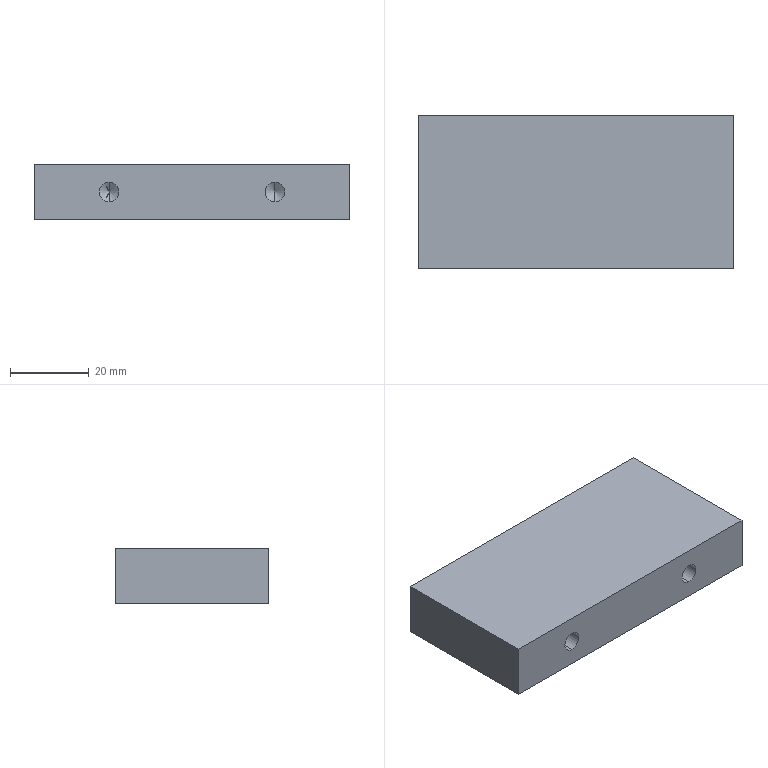Part | SolidWorks | features HoleWzd 2, Extrusion 1 | 1 solid | 22 faces | box 80 x 39 x 14 mm | volume 42305 mm3 | cylinder 8 | cone 8 | plane 6 | commonest cylinder face diameters 5 x8
STEP:
#1=CARTESIAN_POINT('',(-33.,2.5,4.5));
#2=VERTEX_POINT('',#1);
#3=CARTESIAN_POINT('',(-33.,2.5,9.5));
#4=VERTEX_POINT('',#3);
#5=CARTESIAN_POINT('',(-33.,2.5,7.));
#6=DIRECTION('',(0.,1.,0.));
#7=DIRECTION('',(0.,0.,1.));
#8=AXIS2_PLACEMENT_3D('',#5,#6,#7);
#9=CIRCLE('',#8,2.5);
#10=EDGE_CURVE('',#2,#4,#9,.T.);
#11=ORIENTED_EDGE('',*,*,#10,.F.);
#12=CARTESIAN_POINT('',(-33.,19.5,4.5));
#13=VERTEX_POINT('',#12);
#14=CARTESIAN_POINT('',(-33.,19.5,4.5));
#15=DIRECTION('',(0.,1.,0.));
#16=VECTOR('',#15,1000.);
#17=LINE('',#14,#16);
#18=EDGE_CURVE('',#2,#13,#17,.T.);
#19=ORIENTED_EDGE('',*,*,#18,.T.);
#20=CARTESIAN_POINT('',(-33.,19.5,9.5));
#21=VERTEX_POINT('',#20);
#22=CARTESIAN_POINT('',(-33.,19.5,7.));
#23=DIRECTION('',(0.,1.,0.));
#24=DIRECTION('',(0.,0.,1.));
#25=AXIS2_PLACEMENT_3D('',#22,#23,#24);
#26=CIRCLE('',#25,2.5);
#27=EDGE_CURVE('',#13,#21,#26,.T.);
#28=ORIENTED_EDGE('',*,*,#27,.T.);
#29=CARTESIAN_POINT('',(-33.,19.5,9.5));
#30=DIRECTION('',(0.,1.,0.));
#31=VECTOR('',#30,1000.);
#32=LINE('',#29,#31);
#33=EDGE_CURVE('',#4,#21,#32,.T.);
#34=ORIENTED_EDGE('',*,*,#33,.F.);
#35=EDGE_LOOP('',(#11,#19,#28,#34));
#36=FACE_OUTER_BOUND('',#35,.T.);
#37=CARTESIAN_POINT('',(-33.,19.5,7.));
#38=DIRECTION('',(0.,1.,0.));
#39=DIRECTION('',(0.,0.,1.));
#40=AXIS2_PLACEMENT_3D('',#37,#38,#39);
#41=CYLINDRICAL_SURFACE('',#40,2.5);
#42=ADVANCED_FACE('',(#36),#41,.F.);
#43=CARTESIAN_POINT('',(-33.,0.9978,7.));
#44=VERTEX_POINT('',#43);
#45=CARTESIAN_POINT('',(-33.,2.5,9.5));
#46=DIRECTION('',(0.,0.515,0.8572));
#47=VECTOR('',#46,1000.);
#48=LINE('',#45,#47);
#49=EDGE_CURVE('',#44,#4,#48,.T.);
#50=ORIENTED_EDGE('',*,*,#49,.F.);
#51=CARTESIAN_POINT('',(-33.,2.5,4.5));
#52=DIRECTION('',(0.,0.515,-0.8572));
#53=VECTOR('',#52,1000.);
#54=LINE('',#51,#53);
#55=EDGE_CURVE('',#44,#2,#54,.T.);
#56=ORIENTED_EDGE('',*,*,#55,.T.);
#57=ORIENTED_EDGE('',*,*,#10,.T.);
#58=EDGE_LOOP('',(#50,#56,#57));
#59=FACE_OUTER_BOUND('',#58,.T.);
#60=CARTESIAN_POINT('',(-33.,2.5,7.));
#61=DIRECTION('',(0.,1.,0.));
#62=DIRECTION('',(0.,0.,1.));
#63=AXIS2_PLACEMENT_3D('',#60,#61,#62);
#64=CONICAL_SURFACE('',#63,2.5,1.03);
#65=ADVANCED_FACE('',(#59),#64,.F.);
#66=CARTESIAN_POINT('',(33.,2.5,4.5));
#67=VERTEX_POINT('',#66);
#68=CARTESIAN_POINT('',(33.,2.5,9.5));
#69=VERTEX_POINT('',#68);
#70=CARTESIAN_POINT('',(33.,2.5,7.));
#71=DIRECTION('',(0.,1.,0.));
#72=DIRECTION('',(0.,0.,1.));
#73=AXIS2_PLACEMENT_3D('',#70,#71,#72);
#74=CIRCLE('',#73,2.5);
#75=EDGE_CURVE('',#67,#69,#74,.T.);
#76=ORIENTED_EDGE('',*,*,#75,.F.);
#77=CARTESIAN_POINT('',(33.,19.5,4.5));
#78=VERTEX_POINT('',#77);
#79=CARTESIAN_POINT('',(33.,19.5,4.5));
#80=DIRECTION('',(0.,1.,0.));
#81=VECTOR('',#80,1000.);
#82=LINE('',#79,#81);
#83=EDGE_CURVE('',#67,#78,#82,.T.);
#84=ORIENTED_EDGE('',*,*,#83,.T.);
#85=CARTESIAN_POINT('',(33.,19.5,9.5));
#86=VERTEX_POINT('',#85);
#87=CARTESIAN_POINT('',(33.,19.5,7.));
#88=DIRECTION('',(0.,1.,0.));
#89=DIRECTION('',(0.,0.,1.));
#90=AXIS2_PLACEMENT_3D('',#87,#88,#89);
#91=CIRCLE('',#90,2.5);
#92=EDGE_CURVE('',#78,#86,#91,.T.);
#93=ORIENTED_EDGE('',*,*,#92,.T.);
#94=CARTESIAN_POINT('',(33.,19.5,9.5));
#95=DIRECTION('',(0.,1.,0.));
#96=VECTOR('',#95,1000.);
#97=LINE('',#94,#96);
#98=EDGE_CURVE('',#69,#86,#97,.T.);
#99=ORIENTED_EDGE('',*,*,#98,.F.);
#100=EDGE_LOOP('',(#76,#84,#93,#99));
#101=FACE_OUTER_BOUND('',#100,.T.);
#102=CARTESIAN_POINT('',(33.,19.5,7.));
#103=DIRECTION('',(0.,1.,0.));
#104=DIRECTION('',(0.,0.,1.));
#105=AXIS2_PLACEMENT_3D('',#102,#103,#104);
#106=CYLINDRICAL_SURFACE('',#105,2.5);
#107=ADVANCED_FACE('',(#101),#106,.F.);
#108=CARTESIAN_POINT('',(33.,0.9978,7.));
#109=VERTEX_POINT('',#108);
#110=CARTESIAN_POINT('',(33.,2.5,9.5));
#111=DIRECTION('',(0.,0.515,0.8572));
#112=VECTOR('',#111,1000.);
#113=LINE('',#110,#112);
#114=EDGE_CURVE('',#109,#69,#113,.T.);
#115=ORIENTED_EDGE('',*,*,#114,.F.);
#116=CARTESIAN_POINT('',(33.,2.5,4.5));
#117=DIRECTION('',(0.,0.515,-0.8572));
#118=VECTOR('',#117,1000.);
#119=LINE('',#116,#118);
#120=EDGE_CURVE('',#109,#67,#119,.T.);
#121=ORIENTED_EDGE('',*,*,#120,.T.);
#122=ORIENTED_EDGE('',*,*,#75,.T.);
#123=EDGE_LOOP('',(#115,#121,#122));
#124=FACE_OUTER_BOUND('',#123,.T.);
#125=CARTESIAN_POINT('',(33.,2.5,7.));
#126=DIRECTION('',(0.,1.,0.));
#127=DIRECTION('',(0.,0.,1.));
#128=AXIS2_PLACEMENT_3D('',#125,#126,#127);
#129=CONICAL_SURFACE('',#128,2.5,1.03);
#130=ADVANCED_FACE('',(#124),#129,.F.);
#131=CARTESIAN_POINT('',(21.,-2.5,9.5));
#132=VERTEX_POINT('',#131);
#133=CARTESIAN_POINT('',(21.,-2.5,4.5));
#134=VERTEX_POINT('',#133);
#135=CARTESIAN_POINT('',(21.,-2.5,7.));
#136=DIRECTION('',(0.,-1.,0.));
#137=DIRECTION('',(0.,0.,-1.));
#138=AXIS2_PLACEMENT_3D('',#135,#136,#137);
#139=CIRCLE('',#138,2.5);
#140=EDGE_CURVE('',#132,#134,#139,.T.);
#141=ORIENTED_EDGE('',*,*,#140,.F.);
#142=CARTESIAN_POINT('',(21.,-19.5,9.5));
#143=VERTEX_POINT('',#142);
#144=CARTESIAN_POINT('',(21.,-19.5,9.5));
#145=DIRECTION('',(0.,-1.,0.));
#146=VECTOR('',#145,1000.);
#147=LINE('',#144,#146);
#148=EDGE_CURVE('',#132,#143,#147,.T.);
#149=ORIENTED_EDGE('',*,*,#148,.T.);
#150=CARTESIAN_POINT('',(21.,-19.5,4.5));
#151=VERTEX_POINT('',#150);
#152=CARTESIAN_POINT('',(21.,-19.5,7.));
#153=DIRECTION('',(0.,-1.,0.));
#154=DIRECTION('',(0.,0.,-1.));
#155=AXIS2_PLACEMENT_3D('',#152,#153,#154);
#156=CIRCLE('',#155,2.5);
#157=EDGE_CURVE('',#143,#151,#156,.T.);
#158=ORIENTED_EDGE('',*,*,#157,.T.);
#159=CARTESIAN_POINT('',(21.,-19.5,4.5));
#160=DIRECTION('',(0.,-1.,0.));
#161=VECTOR('',#160,1000.);
#162=LINE('',#159,#161);
#163=EDGE_CURVE('',#134,#151,#162,.T.);
#164=ORIENTED_EDGE('',*,*,#163,.F.);
#165=EDGE_LOOP('',(#141,#149,#158,#164));
#166=FACE_OUTER_BOUND('',#165,.T.);
#167=CARTESIAN_POINT('',(21.,-19.5,7.));
#168=DIRECTION('',(0.,-1.,0.));
#169=DIRECTION('',(0.,0.,-1.));
#170=AXIS2_PLACEMENT_3D('',#167,#168,#169);
#171=CYLINDRICAL_SURFACE('',#170,2.5);
#172=ADVANCED_FACE('',(#166),#171,.F.);
#173=CARTESIAN_POINT('',(21.,-0.9978,7.));
#174=VERTEX_POINT('',#173);
#175=CARTESIAN_POINT('',(21.,-2.5,4.5));
#176=DIRECTION('',(0.,-0.515,-0.8572));
#177=VECTOR('',#176,1000.);
#178=LINE('',#175,#177);
#179=EDGE_CURVE('',#174,#134,#178,.T.);
#180=ORIENTED_EDGE('',*,*,#179,.F.);
#181=CARTESIAN_POINT('',(21.,-2.5,9.5));
#182=DIRECTION('',(0.,-0.515,0.8572));
#183=VECTOR('',#182,1000.);
#184=LINE('',#181,#183);
#185=EDGE_CURVE('',#174,#132,#184,.T.);
#186=ORIENTED_EDGE('',*,*,#185,.T.);
#187=ORIENTED_EDGE('',*,*,#140,.T.);
#188=EDGE_LOOP('',(#180,#186,#187));
#189=FACE_OUTER_BOUND('',#188,.T.);
#190=CARTESIAN_POINT('',(21.,-2.5,7.));
#191=DIRECTION('',(0.,-1.,0.));
#192=DIRECTION('',(0.,0.,-1.));
#193=AXIS2_PLACEMENT_3D('',#190,#191,#192);
#194=CONICAL_SURFACE('',#193,2.5,1.03);
#195=ADVANCED_FACE('',(#189),#194,.F.);
#196=CARTESIAN_POINT('',(-21.,-2.5,9.5));
#197=VERTEX_POINT('',#196);
#198=CARTESIAN_POINT('',(-21.,-2.5,4.5));
#199=VERTEX_POINT('',#198);
#200=CARTESIAN_POINT('',(-21.,-2.5,7.));
#201=DIRECTION('',(0.,-1.,0.));
#202=DIRECTION('',(0.,0.,-1.));
#203=AXIS2_PLACEMENT_3D('',#200,#201,#202);
#204=CIRCLE('',#203,2.5);
#205=EDGE_CURVE('',#197,#199,#204,.T.);
#206=ORIENTED_EDGE('',*,*,#205,.F.);
#207=CARTESIAN_POINT('',(-21.,-19.5,9.5));
#208=VERTEX_POINT('',#207);
#209=CARTESIAN_POINT('',(-21.,-19.5,9.5));
#210=DIRECTION('',(0.,-1.,0.));
#211=VECTOR('',#210,1000.);
#212=LINE('',#209,#211);
#213=EDGE_CURVE('',#197,#208,#212,.T.);
#214=ORIENTED_EDGE('',*,*,#213,.T.);
#215=CARTESIAN_POINT('',(-21.,-19.5,4.5));
#216=VERTEX_POINT('',#215);
#217=CARTESIAN_POINT('',(-21.,-19.5,7.));
#218=DIRECTION('',(0.,-1.,0.));
#219=DIRECTION('',(0.,0.,-1.));
#220=AXIS2_PLACEMENT_3D('',#217,#218,#219);
#221=CIRCLE('',#220,2.5);
#222=EDGE_CURVE('',#208,#216,#221,.T.);
#223=ORIENTED_EDGE('',*,*,#222,.T.);
#224=CARTESIAN_POINT('',(-21.,-19.5,4.5));
#225=DIRECTION('',(0.,-1.,0.));
#226=VECTOR('',#225,1000.);
#227=LINE('',#224,#226);
#228=EDGE_CURVE('',#199,#216,#227,.T.);
#229=ORIENTED_EDGE('',*,*,#228,.F.);
#230=EDGE_LOOP('',(#206,#214,#223,#229));
#231=FACE_OUTER_BOUND('',#230,.T.);
#232=CARTESIAN_POINT('',(-21.,-19.5,7.));
#233=DIRECTION('',(0.,-1.,0.));
#234=DIRECTION('',(0.,0.,-1.));
#235=AXIS2_PLACEMENT_3D('',#232,#233,#234);
#236=CYLINDRICAL_SURFACE('',#235,2.5);
#237=ADVANCED_FACE('',(#231),#236,.F.);
#238=CARTESIAN_POINT('',(-21.,-0.9978,7.));
#239=VERTEX_POINT('',#238);
#240=CARTESIAN_POINT('',(-21.,-2.5,4.5));
#241=DIRECTION('',(0.,-0.515,-0.8572));
#242=VECTOR('',#241,1000.);
#243=LINE('',#240,#242);
#244=EDGE_CURVE('',#239,#199,#243,.T.);
#245=ORIENTED_EDGE('',*,*,#244,.F.);
#246=CARTESIAN_POINT('',(-21.,-2.5,9.5));
#247=DIRECTION('',(0.,-0.515,0.8572));
#248=VECTOR('',#247,1000.);
#249=LINE('',#246,#248);
#250=EDGE_CURVE('',#239,#197,#249,.T.);
#251=ORIENTED_EDGE('',*,*,#250,.T.);
#252=ORIENTED_EDGE('',*,*,#205,.T.);
#253=EDGE_LOOP('',(#245,#251,#252));
#254=FACE_OUTER_BOUND('',#253,.T.);
#255=CARTESIAN_POINT('',(-21.,-2.5,7.));
#256=DIRECTION('',(0.,-1.,0.));
#257=DIRECTION('',(0.,0.,-1.));
#258=AXIS2_PLACEMENT_3D('',#255,#256,#257);
#259=CONICAL_SURFACE('',#258,2.5,1.03);
#260=ADVANCED_FACE('',(#254),#259,.F.);
#261=CARTESIAN_POINT('',(40.,-19.5,0.));
#262=VERTEX_POINT('',#261);
#263=CARTESIAN_POINT('',(40.,19.5,0.));
#264=VERTEX_POINT('',#263);
#265=CARTESIAN_POINT('',(40.,19.5,0.));
#266=DIRECTION('',(0.,1.,0.));
#267=VECTOR('',#266,1000.);
#268=LINE('',#265,#267);
#269=EDGE_CURVE('',#262,#264,#268,.T.);
#270=ORIENTED_EDGE('',*,*,#269,.T.);
#271=CARTESIAN_POINT('',(40.,19.5,14.));
#272=VERTEX_POINT('',#271);
#273=CARTESIAN_POINT('',(40.,19.5,14.));
#274=DIRECTION('',(0.,0.,-1.));
#275=VECTOR('',#274,1000.);
#276=LINE('',#273,#275);
#277=EDGE_CURVE('',#272,#264,#276,.T.);
#278=ORIENTED_EDGE('',*,*,#277,.F.);
#279=CARTESIAN_POINT('',(40.,-19.5,14.));
#280=VERTEX_POINT('',#279);
#281=CARTESIAN_POINT('',(40.,19.5,14.));
#282=DIRECTION('',(0.,1.,0.));
#283=VECTOR('',#282,1000.);
#284=LINE('',#281,#283);
#285=EDGE_CURVE('',#280,#272,#284,.T.);
#286=ORIENTED_EDGE('',*,*,#285,.F.);
#287=CARTESIAN_POINT('',(40.,-19.5,14.));
#288=DIRECTION('',(0.,0.,-1.));
#289=VECTOR('',#288,1000.);
#290=LINE('',#287,#289);
#291=EDGE_CURVE('',#280,#262,#290,.T.);
#292=ORIENTED_EDGE('',*,*,#291,.T.);
#293=EDGE_LOOP('',(#270,#278,#286,#292));
#294=FACE_OUTER_BOUND('',#293,.T.);
#295=CARTESIAN_POINT('',(40.,19.5,14.));
#296=DIRECTION('',(-1.,0.,0.));
#297=DIRECTION('',(0.,0.,1.));
#298=AXIS2_PLACEMENT_3D('',#295,#296,#297);
#299=PLANE('',#298);
#300=ADVANCED_FACE('',(#294),#299,.F.);
#301=CARTESIAN_POINT('',(-33.,19.5,7.));
#302=DIRECTION('',(0.,1.,0.));
#303=DIRECTION('',(0.,0.,1.));
#304=AXIS2_PLACEMENT_3D('',#301,#302,#303);
#305=CIRCLE('',#304,2.5);
#306=EDGE_CURVE('',#21,#13,#305,.T.);
#307=ORIENTED_EDGE('',*,*,#306,.F.);
#308=ORIENTED_EDGE('',*,*,#27,.F.);
#309=EDGE_LOOP('',(#307,#308));
#310=FACE_BOUND('',#309,.T.);
#311=CARTESIAN_POINT('',(33.,19.5,7.));
#312=DIRECTION('',(0.,1.,0.));
#313=DIRECTION('',(0.,0.,1.));
#314=AXIS2_PLACEMENT_3D('',#311,#312,#313);
#315=CIRCLE('',#314,2.5);
#316=EDGE_CURVE('',#86,#78,#315,.T.);
#317=ORIENTED_EDGE('',*,*,#316,.F.);
#318=ORIENTED_EDGE('',*,*,#92,.F.);
#319=EDGE_LOOP('',(#317,#318));
#320=FACE_BOUND('',#319,.T.);
#321=CARTESIAN_POINT('',(-40.,19.5,0.));
#322=VERTEX_POINT('',#321);
#323=CARTESIAN_POINT('',(-40.,19.5,0.));
#324=DIRECTION('',(-1.,0.,0.));
#325=VECTOR('',#324,1000.);
#326=LINE('',#323,#325);
#327=EDGE_CURVE('',#264,#322,#326,.T.);
#328=ORIENTED_EDGE('',*,*,#327,.T.);
#329=CARTESIAN_POINT('',(-40.,19.5,14.));
#330=VERTEX_POINT('',#329);
#331=CARTESIAN_POINT('',(-40.,19.5,14.));
#332=DIRECTION('',(0.,0.,-1.));
#333=VECTOR('',#332,1000.);
#334=LINE('',#331,#333);
#335=EDGE_CURVE('',#330,#322,#334,.T.);
#336=ORIENTED_EDGE('',*,*,#335,.F.);
#337=CARTESIAN_POINT('',(-40.,19.5,14.));
#338=DIRECTION('',(-1.,0.,0.));
#339=VECTOR('',#338,1000.);
#340=LINE('',#337,#339);
#341=EDGE_CURVE('',#272,#330,#340,.T.);
#342=ORIENTED_EDGE('',*,*,#341,.F.);
#343=ORIENTED_EDGE('',*,*,#277,.T.);
#344=EDGE_LOOP('',(#328,#336,#342,#343));
#345=FACE_OUTER_BOUND('',#344,.T.);
#346=CARTESIAN_POINT('',(-40.,19.5,14.));
#347=DIRECTION('',(0.,-1.,0.));
#348=DIRECTION('',(0.,0.,-1.));
#349=AXIS2_PLACEMENT_3D('',#346,#347,#348);
#350=PLANE('',#349);
#351=ADVANCED_FACE('',(#310,#320,#345),#350,.F.);
#352=CARTESIAN_POINT('',(-40.,-19.5,0.));
#353=VERTEX_POINT('',#352);
#354=CARTESIAN_POINT('',(-40.,19.5,0.));
#355=DIRECTION('',(0.,-1.,0.));
#356=VECTOR('',#355,1000.);
#357=LINE('',#354,#356);
#358=EDGE_CURVE('',#322,#353,#357,.T.);
#359=ORIENTED_EDGE('',*,*,#358,.T.);
#360=CARTESIAN_POINT('',(-40.,-19.5,14.));
#361=VERTEX_POINT('',#360);
#362=CARTESIAN_POINT('',(-40.,-19.5,14.));
#363=DIRECTION('',(0.,0.,-1.));
#364=VECTOR('',#363,1000.);
#365=LINE('',#362,#364);
#366=EDGE_CURVE('',#361,#353,#365,.T.);
#367=ORIENTED_EDGE('',*,*,#366,.F.);
#368=CARTESIAN_POINT('',(-40.,19.5,14.));
#369=DIRECTION('',(0.,-1.,0.));
#370=VECTOR('',#369,1000.);
#371=LINE('',#368,#370);
#372=EDGE_CURVE('',#330,#361,#371,.T.);
#373=ORIENTED_EDGE('',*,*,#372,.F.);
#374=ORIENTED_EDGE('',*,*,#335,.T.);
#375=EDGE_LOOP('',(#359,#367,#373,#374));
#376=FACE_OUTER_BOUND('',#375,.T.);
#377=CARTESIAN_POINT('',(-40.,19.5,14.));
#378=DIRECTION('',(1.,0.,0.));
#379=DIRECTION('',(0.,1.,0.));
#380=AXIS2_PLACEMENT_3D('',#377,#378,#379);
#381=PLANE('',#380);
#382=ADVANCED_FACE('',(#376),#381,.F.);
#383=CARTESIAN_POINT('',(21.,-19.5,7.));
#384=DIRECTION('',(0.,-1.,0.));
#385=DIRECTION('',(0.,0.,-1.));
#386=AXIS2_PLACEMENT_3D('',#383,#384,#385);
#387=CIRCLE('',#386,2.5);
#388=EDGE_CURVE('',#151,#143,#387,.T.);
#389=ORIENTED_EDGE('',*,*,#388,.F.);
#390=ORIENTED_EDGE('',*,*,#157,.F.);
#391=EDGE_LOOP('',(#389,#390));
#392=FACE_BOUND('',#391,.T.);
#393=CARTESIAN_POINT('',(-21.,-19.5,7.));
#394=DIRECTION('',(0.,-1.,0.));
#395=DIRECTION('',(0.,0.,-1.));
#396=AXIS2_PLACEMENT_3D('',#393,#394,#395);
#397=CIRCLE('',#396,2.5);
#398=EDGE_CURVE('',#216,#208,#397,.T.);
#399=ORIENTED_EDGE('',*,*,#398,.F.);
#400=ORIENTED_EDGE('',*,*,#222,.F.);
#401=EDGE_LOOP('',(#399,#400));
#402=FACE_BOUND('',#401,.T.);
#403=CARTESIAN_POINT('',(-40.,-19.5,0.));
#404=DIRECTION('',(1.,0.,0.));
#405=VECTOR('',#404,1000.);
#406=LINE('',#403,#405);
#407=EDGE_CURVE('',#353,#262,#406,.T.);
#408=ORIENTED_EDGE('',*,*,#407,.T.);
#409=ORIENTED_EDGE('',*,*,#291,.F.);
#410=CARTESIAN_POINT('',(-40.,-19.5,14.));
#411=DIRECTION('',(1.,0.,0.));
#412=VECTOR('',#411,1000.);
#413=LINE('',#410,#412);
#414=EDGE_CURVE('',#361,#280,#413,.T.);
#415=ORIENTED_EDGE('',*,*,#414,.F.);
#416=ORIENTED_EDGE('',*,*,#366,.T.);
#417=EDGE_LOOP('',(#408,#409,#415,#416));
#418=FACE_OUTER_BOUND('',#417,.T.);
#419=CARTESIAN_POINT('',(-40.,-19.5,14.));
#420=DIRECTION('',(0.,1.,0.));
#421=DIRECTION('',(0.,0.,1.));
#422=AXIS2_PLACEMENT_3D('',#419,#420,#421);
#423=PLANE('',#422);
#424=ADVANCED_FACE('',(#392,#402,#418),#423,.F.);
#425=ORIENTED_EDGE('',*,*,#285,.T.);
#426=ORIENTED_EDGE('',*,*,#341,.T.);
#427=ORIENTED_EDGE('',*,*,#372,.T.);
#428=ORIENTED_EDGE('',*,*,#414,.T.);
#429=EDGE_LOOP('',(#425,#426,#427,#428));
#430=FACE_OUTER_BOUND('',#429,.T.);
#431=CARTESIAN_POINT('',(0.,0.,14.));
#432=DIRECTION('',(0.,0.,1.));
#433=DIRECTION('',(1.,0.,0.));
#434=AXIS2_PLACEMENT_3D('',#431,#432,#433);
#435=PLANE('',#434);
#436=ADVANCED_FACE('',(#430),#435,.T.);
#437=ORIENTED_EDGE('',*,*,#269,.F.);
#438=ORIENTED_EDGE('',*,*,#407,.F.);
#439=ORIENTED_EDGE('',*,*,#358,.F.);
#440=ORIENTED_EDGE('',*,*,#327,.F.);
#441=EDGE_LOOP('',(#437,#438,#439,#440));
#442=FACE_OUTER_BOUND('',#441,.T.);
#443=CARTESIAN_POINT('',(0.,0.,0.));
#444=DIRECTION('',(0.,0.,1.));
#445=DIRECTION('',(1.,0.,0.));
#446=AXIS2_PLACEMENT_3D('',#443,#444,#445);
#447=PLANE('',#446);
#448=ADVANCED_FACE('',(#442),#447,.F.);
#449=ORIENTED_EDGE('',*,*,#250,.F.);
#450=ORIENTED_EDGE('',*,*,#244,.T.);
#451=CARTESIAN_POINT('',(-21.,-2.5,7.));
#452=DIRECTION('',(0.,-1.,0.));
#453=DIRECTION('',(0.,0.,-1.));
#454=AXIS2_PLACEMENT_3D('',#451,#452,#453);
#455=CIRCLE('',#454,2.5);
#456=EDGE_CURVE('',#199,#197,#455,.T.);
#457=ORIENTED_EDGE('',*,*,#456,.T.);
#458=EDGE_LOOP('',(#449,#450,#457));
#459=FACE_OUTER_BOUND('',#458,.T.);
#460=CARTESIAN_POINT('',(-21.,-2.5,7.));
#461=DIRECTION('',(0.,-1.,0.));
#462=DIRECTION('',(0.,0.,-1.));
#463=AXIS2_PLACEMENT_3D('',#460,#461,#462);
#464=CONICAL_SURFACE('',#463,2.5,1.03);
#465=ADVANCED_FACE('',(#459),#464,.F.);
#466=ORIENTED_EDGE('',*,*,#213,.F.);
#467=ORIENTED_EDGE('',*,*,#456,.F.);
#468=ORIENTED_EDGE('',*,*,#228,.T.);
#469=ORIENTED_EDGE('',*,*,#398,.T.);
#470=EDGE_LOOP('',(#466,#467,#468,#469));
#471=FACE_OUTER_BOUND('',#470,.T.);
#472=CARTESIAN_POINT('',(-21.,-19.5,7.));
#473=DIRECTION('',(0.,-1.,0.));
#474=DIRECTION('',(0.,0.,-1.));
#475=AXIS2_PLACEMENT_3D('',#472,#473,#474);
#476=CYLINDRICAL_SURFACE('',#475,2.5);
#477=ADVANCED_FACE('',(#471),#476,.F.);
#478=ORIENTED_EDGE('',*,*,#185,.F.);
#479=ORIENTED_EDGE('',*,*,#179,.T.);
#480=CARTESIAN_POINT('',(21.,-2.5,7.));
#481=DIRECTION('',(0.,-1.,0.));
#482=DIRECTION('',(0.,0.,-1.));
#483=AXIS2_PLACEMENT_3D('',#480,#481,#482);
#484=CIRCLE('',#483,2.5);
#485=EDGE_CURVE('',#134,#132,#484,.T.);
#486=ORIENTED_EDGE('',*,*,#485,.T.);
#487=EDGE_LOOP('',(#478,#479,#486));
#488=FACE_OUTER_BOUND('',#487,.T.);
#489=CARTESIAN_POINT('',(21.,-2.5,7.));
#490=DIRECTION('',(0.,-1.,0.));
#491=DIRECTION('',(0.,0.,-1.));
#492=AXIS2_PLACEMENT_3D('',#489,#490,#491);
#493=CONICAL_SURFACE('',#492,2.5,1.03);
#494=ADVANCED_FACE('',(#488),#493,.F.);
#495=ORIENTED_EDGE('',*,*,#148,.F.);
#496=ORIENTED_EDGE('',*,*,#485,.F.);
#497=ORIENTED_EDGE('',*,*,#163,.T.);
#498=ORIENTED_EDGE('',*,*,#388,.T.);
#499=EDGE_LOOP('',(#495,#496,#497,#498));
#500=FACE_OUTER_BOUND('',#499,.T.);
#501=CARTESIAN_POINT('',(21.,-19.5,7.));
#502=DIRECTION('',(0.,-1.,0.));
#503=DIRECTION('',(0.,0.,-1.));
#504=AXIS2_PLACEMENT_3D('',#501,#502,#503);
#505=CYLINDRICAL_SURFACE('',#504,2.5);
#506=ADVANCED_FACE('',(#500),#505,.F.);
#507=ORIENTED_EDGE('',*,*,#120,.F.);
#508=ORIENTED_EDGE('',*,*,#114,.T.);
#509=CARTESIAN_POINT('',(33.,2.5,7.));
#510=DIRECTION('',(0.,1.,0.));
#511=DIRECTION('',(0.,0.,1.));
#512=AXIS2_PLACEMENT_3D('',#509,#510,#511);
#513=CIRCLE('',#512,2.5);
#514=EDGE_CURVE('',#69,#67,#513,.T.);
#515=ORIENTED_EDGE('',*,*,#514,.T.);
#516=EDGE_LOOP('',(#507,#508,#515));
#517=FACE_OUTER_BOUND('',#516,.T.);
#518=CARTESIAN_POINT('',(33.,2.5,7.));
#519=DIRECTION('',(0.,1.,0.));
#520=DIRECTION('',(0.,0.,1.));
#521=AXIS2_PLACEMENT_3D('',#518,#519,#520);
#522=CONICAL_SURFACE('',#521,2.5,1.03);
#523=ADVANCED_FACE('',(#517),#522,.F.);
#524=ORIENTED_EDGE('',*,*,#83,.F.);
#525=ORIENTED_EDGE('',*,*,#514,.F.);
#526=ORIENTED_EDGE('',*,*,#98,.T.);
#527=ORIENTED_EDGE('',*,*,#316,.T.);
#528=EDGE_LOOP('',(#524,#525,#526,#527));
#529=FACE_OUTER_BOUND('',#528,.T.);
#530=CARTESIAN_POINT('',(33.,19.5,7.));
#531=DIRECTION('',(0.,1.,0.));
#532=DIRECTION('',(0.,0.,1.));
#533=AXIS2_PLACEMENT_3D('',#530,#531,#532);
#534=CYLINDRICAL_SURFACE('',#533,2.5);
#535=ADVANCED_FACE('',(#529),#534,.F.);
#536=ORIENTED_EDGE('',*,*,#55,.F.);
#537=ORIENTED_EDGE('',*,*,#49,.T.);
#538=CARTESIAN_POINT('',(-33.,2.5,7.));
#539=DIRECTION('',(0.,1.,0.));
#540=DIRECTION('',(0.,0.,1.));
#541=AXIS2_PLACEMENT_3D('',#538,#539,#540);
#542=CIRCLE('',#541,2.5);
#543=EDGE_CURVE('',#4,#2,#542,.T.);
#544=ORIENTED_EDGE('',*,*,#543,.T.);
#545=EDGE_LOOP('',(#536,#537,#544));
#546=FACE_OUTER_BOUND('',#545,.T.);
#547=CARTESIAN_POINT('',(-33.,2.5,7.));
#548=DIRECTION('',(0.,1.,0.));
#549=DIRECTION('',(0.,0.,1.));
#550=AXIS2_PLACEMENT_3D('',#547,#548,#549);
#551=CONICAL_SURFACE('',#550,2.5,1.03);
#552=ADVANCED_FACE('',(#546),#551,.F.);
#553=ORIENTED_EDGE('',*,*,#18,.F.);
#554=ORIENTED_EDGE('',*,*,#543,.F.);
#555=ORIENTED_EDGE('',*,*,#33,.T.);
#556=ORIENTED_EDGE('',*,*,#306,.T.);
#557=EDGE_LOOP('',(#553,#554,#555,#556));
#558=FACE_OUTER_BOUND('',#557,.T.);
#559=CARTESIAN_POINT('',(-33.,19.5,7.));
#560=DIRECTION('',(0.,1.,0.));
#561=DIRECTION('',(0.,0.,1.));
#562=AXIS2_PLACEMENT_3D('',#559,#560,#561);
#563=CYLINDRICAL_SURFACE('',#562,2.5);
#564=ADVANCED_FACE('',(#558),#563,.F.);
#565=CLOSED_SHELL('',(#42,#65,#107,#130,#172,#195,#237,#260,#300,#351,#382,#424,#436,#448,#465,#477,#494,#506,#523,#535,#552,#564));
#566=MANIFOLD_SOLID_BREP('',#565);
#567=CARTESIAN_POINT('',(0.,0.,0.));
#568=DIRECTION('',(0.,0.,1.));
#569=DIRECTION('',(1.,0.,0.));
#570=AXIS2_PLACEMENT_3D('',#567,#568,#569);
#571=(LENGTH_UNIT()NAMED_UNIT(*)SI_UNIT(.MILLI.,.METRE.));
#572=UNCERTAINTY_MEASURE_WITH_UNIT(LENGTH_MEASURE(0.00001),#571,'','');
#573=(NAMED_UNIT(*)PLANE_ANGLE_UNIT()SI_UNIT($,.RADIAN.));
#574=(NAMED_UNIT(*)SI_UNIT($,.STERADIAN.)SOLID_ANGLE_UNIT());
#575=(GEOMETRIC_REPRESENTATION_CONTEXT(3)GLOBAL_UNCERTAINTY_ASSIGNED_CONTEXT((#572))GLOBAL_UNIT_ASSIGNED_CONTEXT((#571,#573,#574))REPRESENTATION_CONTEXT('',''));
#576=ADVANCED_BREP_SHAPE_REPRESENTATION('',(#566,#570),#575);